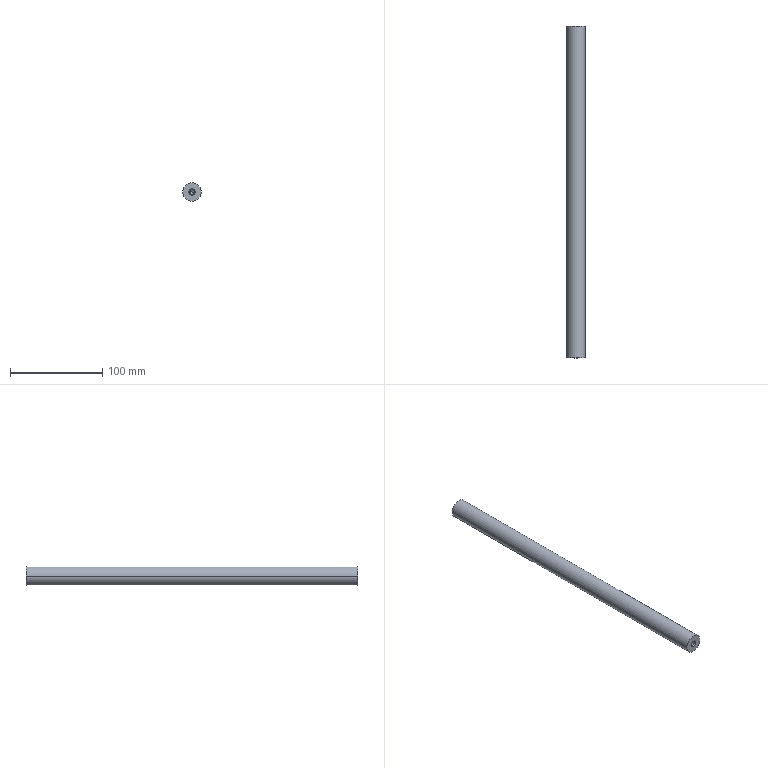Part | NX | features BREP 1 | 1 solid | 16 faces | box 20 x 360 x 20 mm | volume 112302 mm3 | cone 8 | cylinder 6 | plane 2 | commonest cylinder face diameters 4.917 x4 20 x2
STEP:
#1=CARTESIAN_POINT('',(10.,-180.,0.));
#2=VERTEX_POINT('',#1);
#3=CARTESIAN_POINT('',(-10.,-180.,0.));
#4=VERTEX_POINT('',#3);
#5=CARTESIAN_POINT('',(0.,-180.,0.));
#6=DIRECTION('',(0.,-1.,0.));
#7=DIRECTION('',(1.,0.,0.));
#8=AXIS2_PLACEMENT_3D('',#5,#6,#7);
#9=CIRCLE('',#8,10.);
#10=EDGE_CURVE('',#2,#4,#9,.T.);
#11=ORIENTED_EDGE('',*,*,#10,.T.);
#12=CARTESIAN_POINT('',(0.,-180.,0.));
#13=DIRECTION('',(0.,-1.,0.));
#14=DIRECTION('',(-1.,0.,0.));
#15=AXIS2_PLACEMENT_3D('',#12,#13,#14);
#16=CIRCLE('',#15,10.);
#17=EDGE_CURVE('',#4,#2,#16,.T.);
#18=ORIENTED_EDGE('',*,*,#17,.T.);
#19=EDGE_LOOP('',(#11,#18));
#20=FACE_BOUND('',#19,.T.);
#21=CARTESIAN_POINT('',(-3.458,-180.,0.));
#22=VERTEX_POINT('',#21);
#23=CARTESIAN_POINT('',(3.458,-180.,0.));
#24=VERTEX_POINT('',#23);
#25=CARTESIAN_POINT('',(0.,-180.,0.));
#26=DIRECTION('',(0.,1.,0.));
#27=DIRECTION('',(-1.,0.,0.));
#28=AXIS2_PLACEMENT_3D('',#25,#26,#27);
#29=CIRCLE('',#28,3.458);
#30=EDGE_CURVE('',#22,#24,#29,.T.);
#31=ORIENTED_EDGE('',*,*,#30,.T.);
#32=CARTESIAN_POINT('',(0.,-180.,0.));
#33=DIRECTION('',(0.,1.,0.));
#34=DIRECTION('',(1.,0.,0.));
#35=AXIS2_PLACEMENT_3D('',#32,#33,#34);
#36=CIRCLE('',#35,3.458);
#37=EDGE_CURVE('',#24,#22,#36,.T.);
#38=ORIENTED_EDGE('',*,*,#37,.T.);
#39=EDGE_LOOP('',(#31,#38));
#40=FACE_BOUND('',#39,.T.);
#41=CARTESIAN_POINT('',(0.,-180.,0.));
#42=DIRECTION('',(0.,1.,0.));
#43=DIRECTION('',(1.,0.,0.));
#44=AXIS2_PLACEMENT_3D('',#41,#42,#43);
#45=PLANE('',#44);
#46=ADVANCED_FACE('',(#20,#40),#45,.F.);
#47=ORIENTED_EDGE('',*,*,#17,.F.);
#48=CARTESIAN_POINT('',(-10.,180.,0.));
#49=VERTEX_POINT('',#48);
#50=CARTESIAN_POINT('',(-10.,180.,0.));
#51=DIRECTION('',(0.,-1.,0.));
#52=VECTOR('',#51,1000.);
#53=LINE('',#50,#52);
#54=EDGE_CURVE('',#49,#4,#53,.T.);
#55=ORIENTED_EDGE('',*,*,#54,.F.);
#56=CARTESIAN_POINT('',(10.,180.,0.));
#57=VERTEX_POINT('',#56);
#58=CARTESIAN_POINT('',(0.,180.,0.));
#59=DIRECTION('',(0.,1.,0.));
#60=DIRECTION('',(1.,0.,0.));
#61=AXIS2_PLACEMENT_3D('',#58,#59,#60);
#62=CIRCLE('',#61,10.);
#63=EDGE_CURVE('',#57,#49,#62,.T.);
#64=ORIENTED_EDGE('',*,*,#63,.F.);
#65=CARTESIAN_POINT('',(10.,180.,0.));
#66=DIRECTION('',(0.,-1.,0.));
#67=VECTOR('',#66,1000.);
#68=LINE('',#65,#67);
#69=EDGE_CURVE('',#57,#2,#68,.T.);
#70=ORIENTED_EDGE('',*,*,#69,.T.);
#71=EDGE_LOOP('',(#47,#55,#64,#70));
#72=FACE_BOUND('',#71,.T.);
#73=CARTESIAN_POINT('',(0.,0.,0.));
#74=DIRECTION('',(0.,1.,0.));
#75=DIRECTION('',(-1.,0.,0.));
#76=AXIS2_PLACEMENT_3D('',#73,#74,#75);
#77=CYLINDRICAL_SURFACE('',#76,10.);
#78=ADVANCED_FACE('',(#72),#77,.T.);
#79=ORIENTED_EDGE('',*,*,#10,.F.);
#80=ORIENTED_EDGE('',*,*,#69,.F.);
#81=CARTESIAN_POINT('',(0.,180.,0.));
#82=DIRECTION('',(0.,1.,0.));
#83=DIRECTION('',(-1.,0.,0.));
#84=AXIS2_PLACEMENT_3D('',#81,#82,#83);
#85=CIRCLE('',#84,10.);
#86=EDGE_CURVE('',#49,#57,#85,.T.);
#87=ORIENTED_EDGE('',*,*,#86,.F.);
#88=ORIENTED_EDGE('',*,*,#54,.T.);
#89=EDGE_LOOP('',(#79,#80,#87,#88));
#90=FACE_BOUND('',#89,.T.);
#91=CARTESIAN_POINT('',(0.,0.,0.));
#92=DIRECTION('',(0.,1.,0.));
#93=DIRECTION('',(-1.,0.,0.));
#94=AXIS2_PLACEMENT_3D('',#91,#92,#93);
#95=CYLINDRICAL_SURFACE('',#94,10.);
#96=ADVANCED_FACE('',(#90),#95,.T.);
#97=ORIENTED_EDGE('',*,*,#63,.T.);
#98=ORIENTED_EDGE('',*,*,#86,.T.);
#99=EDGE_LOOP('',(#97,#98));
#100=FACE_BOUND('',#99,.T.);
#101=CARTESIAN_POINT('',(3.458,180.,0.));
#102=VERTEX_POINT('',#101);
#103=CARTESIAN_POINT('',(-3.458,180.,0.));
#104=VERTEX_POINT('',#103);
#105=CARTESIAN_POINT('',(0.,180.,0.));
#106=DIRECTION('',(0.,-1.,0.));
#107=DIRECTION('',(1.,0.,0.));
#108=AXIS2_PLACEMENT_3D('',#105,#106,#107);
#109=CIRCLE('',#108,3.458);
#110=EDGE_CURVE('',#102,#104,#109,.T.);
#111=ORIENTED_EDGE('',*,*,#110,.T.);
#112=CARTESIAN_POINT('',(0.,180.,0.));
#113=DIRECTION('',(0.,-1.,0.));
#114=DIRECTION('',(-1.,0.,0.));
#115=AXIS2_PLACEMENT_3D('',#112,#113,#114);
#116=CIRCLE('',#115,3.458);
#117=EDGE_CURVE('',#104,#102,#116,.T.);
#118=ORIENTED_EDGE('',*,*,#117,.T.);
#119=EDGE_LOOP('',(#111,#118));
#120=FACE_BOUND('',#119,.T.);
#121=CARTESIAN_POINT('',(0.,180.,0.));
#122=DIRECTION('',(0.,1.,0.));
#123=DIRECTION('',(1.,0.,0.));
#124=AXIS2_PLACEMENT_3D('',#121,#122,#123);
#125=PLANE('',#124);
#126=ADVANCED_FACE('',(#100,#120),#125,.T.);
#127=ORIENTED_EDGE('',*,*,#117,.F.);
#128=CARTESIAN_POINT('',(-2.458,179.,0.));
#129=VERTEX_POINT('',#128);
#130=CARTESIAN_POINT('',(-3.458,180.,0.));
#131=DIRECTION('',(0.7071,-0.7071,0.));
#132=VECTOR('',#131,1000.);
#133=LINE('',#130,#132);
#134=EDGE_CURVE('',#129,#104,#133,.F.);
#135=ORIENTED_EDGE('',*,*,#134,.F.);
#136=CARTESIAN_POINT('',(2.458,179.,0.));
#137=VERTEX_POINT('',#136);
#138=CARTESIAN_POINT('',(0.,179.,0.));
#139=DIRECTION('',(0.,-1.,0.));
#140=DIRECTION('',(-1.,0.,0.));
#141=AXIS2_PLACEMENT_3D('',#138,#139,#140);
#142=CIRCLE('',#141,2.458);
#143=EDGE_CURVE('',#129,#137,#142,.T.);
#144=ORIENTED_EDGE('',*,*,#143,.T.);
#145=CARTESIAN_POINT('',(3.458,180.,0.));
#146=DIRECTION('',(-0.7071,-0.7071,0.));
#147=VECTOR('',#146,1000.);
#148=LINE('',#145,#147);
#149=EDGE_CURVE('',#137,#102,#148,.F.);
#150=ORIENTED_EDGE('',*,*,#149,.T.);
#151=EDGE_LOOP('',(#127,#135,#144,#150));
#152=FACE_BOUND('',#151,.T.);
#153=CARTESIAN_POINT('',(0.,179.5,0.));
#154=DIRECTION('',(0.,1.,0.));
#155=DIRECTION('',(1.,0.,0.));
#156=AXIS2_PLACEMENT_3D('',#153,#154,#155);
#157=CONICAL_SURFACE('',#156,2.958,0.7854);
#158=ADVANCED_FACE('',(#152),#157,.F.);
#159=ORIENTED_EDGE('',*,*,#134,.T.);
#160=ORIENTED_EDGE('',*,*,#110,.F.);
#161=ORIENTED_EDGE('',*,*,#149,.F.);
#162=CARTESIAN_POINT('',(0.,179.,0.));
#163=DIRECTION('',(0.,-1.,0.));
#164=DIRECTION('',(1.,0.,0.));
#165=AXIS2_PLACEMENT_3D('',#162,#163,#164);
#166=CIRCLE('',#165,2.458);
#167=EDGE_CURVE('',#137,#129,#166,.T.);
#168=ORIENTED_EDGE('',*,*,#167,.T.);
#169=EDGE_LOOP('',(#159,#160,#161,#168));
#170=FACE_BOUND('',#169,.T.);
#171=CARTESIAN_POINT('',(0.,179.5,0.));
#172=DIRECTION('',(0.,1.,0.));
#173=DIRECTION('',(-0.5,0.,-0.866));
#174=AXIS2_PLACEMENT_3D('',#171,#172,#173);
#175=CONICAL_SURFACE('',#174,2.958,0.7854);
#176=ADVANCED_FACE('',(#170),#175,.F.);
#177=ORIENTED_EDGE('',*,*,#167,.F.);
#178=CARTESIAN_POINT('',(2.459,160.,0.));
#179=VERTEX_POINT('',#178);
#180=CARTESIAN_POINT('',(2.458,179.,0.));
#181=DIRECTION('',(0.,-1.,0.));
#182=VECTOR('',#181,1000.);
#183=LINE('',#180,#182);
#184=EDGE_CURVE('',#179,#137,#183,.F.);
#185=ORIENTED_EDGE('',*,*,#184,.F.);
#186=CARTESIAN_POINT('',(-2.459,160.,0.));
#187=VERTEX_POINT('',#186);
#188=CARTESIAN_POINT('',(0.,160.,0.));
#189=DIRECTION('',(0.,1.,0.));
#190=DIRECTION('',(-1.,0.,0.));
#191=AXIS2_PLACEMENT_3D('',#188,#189,#190);
#192=CIRCLE('',#191,2.459);
#193=EDGE_CURVE('',#187,#179,#192,.T.);
#194=ORIENTED_EDGE('',*,*,#193,.F.);
#195=CARTESIAN_POINT('',(-2.458,179.,0.));
#196=DIRECTION('',(0.,-1.,0.));
#197=VECTOR('',#196,1000.);
#198=LINE('',#195,#197);
#199=EDGE_CURVE('',#187,#129,#198,.F.);
#200=ORIENTED_EDGE('',*,*,#199,.T.);
#201=EDGE_LOOP('',(#177,#185,#194,#200));
#202=FACE_BOUND('',#201,.T.);
#203=CARTESIAN_POINT('',(0.,180.,0.));
#204=DIRECTION('',(0.,-1.,0.));
#205=DIRECTION('',(1.,0.,0.));
#206=AXIS2_PLACEMENT_3D('',#203,#204,#205);
#207=CYLINDRICAL_SURFACE('',#206,2.458);
#208=ADVANCED_FACE('',(#202),#207,.F.);
#209=ORIENTED_EDGE('',*,*,#199,.F.);
#210=CARTESIAN_POINT('',(0.,160.,0.));
#211=DIRECTION('',(0.,1.,0.));
#212=DIRECTION('',(1.,0.,0.));
#213=AXIS2_PLACEMENT_3D('',#210,#211,#212);
#214=CIRCLE('',#213,2.459);
#215=EDGE_CURVE('',#179,#187,#214,.T.);
#216=ORIENTED_EDGE('',*,*,#215,.F.);
#217=ORIENTED_EDGE('',*,*,#184,.T.);
#218=ORIENTED_EDGE('',*,*,#143,.F.);
#219=EDGE_LOOP('',(#209,#216,#217,#218));
#220=FACE_BOUND('',#219,.T.);
#221=CARTESIAN_POINT('',(0.,180.,0.));
#222=DIRECTION('',(0.,-1.,0.));
#223=DIRECTION('',(1.,0.,0.));
#224=AXIS2_PLACEMENT_3D('',#221,#222,#223);
#225=CYLINDRICAL_SURFACE('',#224,2.458);
#226=ADVANCED_FACE('',(#220),#225,.F.);
#227=ORIENTED_EDGE('',*,*,#215,.T.);
#228=CARTESIAN_POINT('',(0.,158.581,0.));
#229=VERTEX_POINT('',#228);
#230=CARTESIAN_POINT('',(-2.459,160.,0.));
#231=DIRECTION('',(0.866,-0.5,0.));
#232=VECTOR('',#231,1000.);
#233=LINE('',#230,#232);
#234=EDGE_CURVE('',#187,#229,#233,.T.);
#235=ORIENTED_EDGE('',*,*,#234,.T.);
#236=CARTESIAN_POINT('',(2.459,160.,0.));
#237=DIRECTION('',(-0.866,-0.5,0.));
#238=VECTOR('',#237,1000.);
#239=LINE('',#236,#238);
#240=EDGE_CURVE('',#179,#229,#239,.T.);
#241=ORIENTED_EDGE('',*,*,#240,.F.);
#242=EDGE_LOOP('',(#227,#235,#241));
#243=FACE_BOUND('',#242,.T.);
#244=CARTESIAN_POINT('',(0.,159.399,0.));
#245=DIRECTION('',(0.,1.,0.));
#246=DIRECTION('',(1.,0.,0.));
#247=AXIS2_PLACEMENT_3D('',#244,#245,#246);
#248=CONICAL_SURFACE('',#247,1.417,1.047);
#249=ADVANCED_FACE('',(#243),#248,.F.);
#250=ORIENTED_EDGE('',*,*,#193,.T.);
#251=ORIENTED_EDGE('',*,*,#240,.T.);
#252=ORIENTED_EDGE('',*,*,#234,.F.);
#253=EDGE_LOOP('',(#250,#251,#252));
#254=FACE_BOUND('',#253,.T.);
#255=CARTESIAN_POINT('',(0.,159.399,0.));
#256=DIRECTION('',(0.,1.,0.));
#257=DIRECTION('',(1.,0.,0.));
#258=AXIS2_PLACEMENT_3D('',#255,#256,#257);
#259=CONICAL_SURFACE('',#258,1.417,1.047);
#260=ADVANCED_FACE('',(#254),#259,.F.);
#261=CARTESIAN_POINT('',(-2.458,-179.,0.));
#262=VERTEX_POINT('',#261);
#263=CARTESIAN_POINT('',(-3.458,-180.,0.));
#264=DIRECTION('',(0.7071,0.7071,0.));
#265=VECTOR('',#264,1000.);
#266=LINE('',#263,#265);
#267=EDGE_CURVE('',#22,#262,#266,.T.);
#268=ORIENTED_EDGE('',*,*,#267,.F.);
#269=ORIENTED_EDGE('',*,*,#37,.F.);
#270=CARTESIAN_POINT('',(2.458,-179.,0.));
#271=VERTEX_POINT('',#270);
#272=CARTESIAN_POINT('',(3.458,-180.,0.));
#273=DIRECTION('',(-0.7071,0.7071,0.));
#274=VECTOR('',#273,1000.);
#275=LINE('',#272,#274);
#276=EDGE_CURVE('',#24,#271,#275,.T.);
#277=ORIENTED_EDGE('',*,*,#276,.T.);
#278=CARTESIAN_POINT('',(0.,-179.,0.));
#279=DIRECTION('',(0.,1.,0.));
#280=DIRECTION('',(1.,0.,0.));
#281=AXIS2_PLACEMENT_3D('',#278,#279,#280);
#282=CIRCLE('',#281,2.458);
#283=EDGE_CURVE('',#271,#262,#282,.T.);
#284=ORIENTED_EDGE('',*,*,#283,.T.);
#285=EDGE_LOOP('',(#268,#269,#277,#284));
#286=FACE_BOUND('',#285,.T.);
#287=CARTESIAN_POINT('',(0.,-179.5,0.));
#288=DIRECTION('',(0.,-1.,0.));
#289=DIRECTION('',(1.,0.,0.));
#290=AXIS2_PLACEMENT_3D('',#287,#288,#289);
#291=CONICAL_SURFACE('',#290,2.958,0.7854);
#292=ADVANCED_FACE('',(#286),#291,.F.);
#293=CARTESIAN_POINT('',(2.459,-160.,0.));
#294=VERTEX_POINT('',#293);
#295=CARTESIAN_POINT('',(2.458,-179.,0.));
#296=DIRECTION('',(0.,1.,0.));
#297=VECTOR('',#296,1000.);
#298=LINE('',#295,#297);
#299=EDGE_CURVE('',#294,#271,#298,.F.);
#300=ORIENTED_EDGE('',*,*,#299,.F.);
#301=CARTESIAN_POINT('',(-2.459,-160.,0.));
#302=VERTEX_POINT('',#301);
#303=CARTESIAN_POINT('',(0.,-160.,0.));
#304=DIRECTION('',(0.,-1.,0.));
#305=DIRECTION('',(-1.,0.,0.));
#306=AXIS2_PLACEMENT_3D('',#303,#304,#305);
#307=CIRCLE('',#306,2.459);
#308=EDGE_CURVE('',#302,#294,#307,.T.);
#309=ORIENTED_EDGE('',*,*,#308,.F.);
#310=CARTESIAN_POINT('',(-2.458,-179.,0.));
#311=DIRECTION('',(0.,1.,0.));
#312=VECTOR('',#311,1000.);
#313=LINE('',#310,#312);
#314=EDGE_CURVE('',#302,#262,#313,.F.);
#315=ORIENTED_EDGE('',*,*,#314,.T.);
#316=ORIENTED_EDGE('',*,*,#283,.F.);
#317=EDGE_LOOP('',(#300,#309,#315,#316));
#318=FACE_BOUND('',#317,.T.);
#319=CARTESIAN_POINT('',(0.,180.,0.));
#320=DIRECTION('',(0.,-1.,0.));
#321=DIRECTION('',(1.,0.,0.));
#322=AXIS2_PLACEMENT_3D('',#319,#320,#321);
#323=CYLINDRICAL_SURFACE('',#322,2.458);
#324=ADVANCED_FACE('',(#318),#323,.F.);
#325=CARTESIAN_POINT('',(0.,-179.,0.));
#326=DIRECTION('',(0.,1.,0.));
#327=DIRECTION('',(-1.,0.,0.));
#328=AXIS2_PLACEMENT_3D('',#325,#326,#327);
#329=CIRCLE('',#328,2.458);
#330=EDGE_CURVE('',#262,#271,#329,.T.);
#331=ORIENTED_EDGE('',*,*,#330,.F.);
#332=ORIENTED_EDGE('',*,*,#314,.F.);
#333=CARTESIAN_POINT('',(0.,-160.,0.));
#334=DIRECTION('',(0.,-1.,0.));
#335=DIRECTION('',(1.,0.,0.));
#336=AXIS2_PLACEMENT_3D('',#333,#334,#335);
#337=CIRCLE('',#336,2.459);
#338=EDGE_CURVE('',#294,#302,#337,.T.);
#339=ORIENTED_EDGE('',*,*,#338,.F.);
#340=ORIENTED_EDGE('',*,*,#299,.T.);
#341=EDGE_LOOP('',(#331,#332,#339,#340));
#342=FACE_BOUND('',#341,.T.);
#343=CARTESIAN_POINT('',(0.,180.,0.));
#344=DIRECTION('',(0.,-1.,0.));
#345=DIRECTION('',(1.,0.,0.));
#346=AXIS2_PLACEMENT_3D('',#343,#344,#345);
#347=CYLINDRICAL_SURFACE('',#346,2.458);
#348=ADVANCED_FACE('',(#342),#347,.F.);
#349=ORIENTED_EDGE('',*,*,#330,.T.);
#350=ORIENTED_EDGE('',*,*,#276,.F.);
#351=ORIENTED_EDGE('',*,*,#30,.F.);
#352=ORIENTED_EDGE('',*,*,#267,.T.);
#353=EDGE_LOOP('',(#349,#350,#351,#352));
#354=FACE_BOUND('',#353,.T.);
#355=CARTESIAN_POINT('',(0.,-179.5,0.));
#356=DIRECTION('',(0.,-1.,0.));
#357=DIRECTION('',(-0.5,0.,-0.866));
#358=AXIS2_PLACEMENT_3D('',#355,#356,#357);
#359=CONICAL_SURFACE('',#358,2.958,0.7854);
#360=ADVANCED_FACE('',(#354),#359,.F.);
#361=ORIENTED_EDGE('',*,*,#338,.T.);
#362=CARTESIAN_POINT('',(0.,-158.581,0.));
#363=VERTEX_POINT('',#362);
#364=CARTESIAN_POINT('',(-2.459,-160.,0.));
#365=DIRECTION('',(0.866,0.5,0.));
#366=VECTOR('',#365,1000.);
#367=LINE('',#364,#366);
#368=EDGE_CURVE('',#302,#363,#367,.T.);
#369=ORIENTED_EDGE('',*,*,#368,.T.);
#370=CARTESIAN_POINT('',(2.459,-160.,0.));
#371=DIRECTION('',(-0.866,0.5,0.));
#372=VECTOR('',#371,1000.);
#373=LINE('',#370,#372);
#374=EDGE_CURVE('',#294,#363,#373,.T.);
#375=ORIENTED_EDGE('',*,*,#374,.F.);
#376=EDGE_LOOP('',(#361,#369,#375));
#377=FACE_BOUND('',#376,.T.);
#378=CARTESIAN_POINT('',(0.,-159.399,0.));
#379=DIRECTION('',(0.,-1.,0.));
#380=DIRECTION('',(1.,0.,0.));
#381=AXIS2_PLACEMENT_3D('',#378,#379,#380);
#382=CONICAL_SURFACE('',#381,1.417,1.047);
#383=ADVANCED_FACE('',(#377),#382,.F.);
#384=ORIENTED_EDGE('',*,*,#308,.T.);
#385=ORIENTED_EDGE('',*,*,#374,.T.);
#386=ORIENTED_EDGE('',*,*,#368,.F.);
#387=EDGE_LOOP('',(#384,#385,#386));
#388=FACE_BOUND('',#387,.T.);
#389=CARTESIAN_POINT('',(0.,-159.399,0.));
#390=DIRECTION('',(0.,-1.,0.));
#391=DIRECTION('',(1.,0.,0.));
#392=AXIS2_PLACEMENT_3D('',#389,#390,#391);
#393=CONICAL_SURFACE('',#392,1.417,1.047);
#394=ADVANCED_FACE('',(#388),#393,.F.);
#395=CLOSED_SHELL('',(#46,#78,#96,#126,#158,#176,#208,#226,#249,#260,#292,#324,#348,#360,#383,#394));
#396=MANIFOLD_SOLID_BREP('',#395);
#397=(LENGTH_UNIT()NAMED_UNIT(*)SI_UNIT(.MILLI.,.METRE.));
#398=UNCERTAINTY_MEASURE_WITH_UNIT(LENGTH_MEASURE(0.00001),#397,'','');
#399=(NAMED_UNIT(*)PLANE_ANGLE_UNIT()SI_UNIT($,.RADIAN.));
#400=(NAMED_UNIT(*)SI_UNIT($,.STERADIAN.)SOLID_ANGLE_UNIT());
#401=(GEOMETRIC_REPRESENTATION_CONTEXT(3)GLOBAL_UNCERTAINTY_ASSIGNED_CONTEXT((#398))GLOBAL_UNIT_ASSIGNED_CONTEXT((#397,#399,#400))REPRESENTATION_CONTEXT('',''));
#402=ADVANCED_BREP_SHAPE_REPRESENTATION('',(#396),#401);